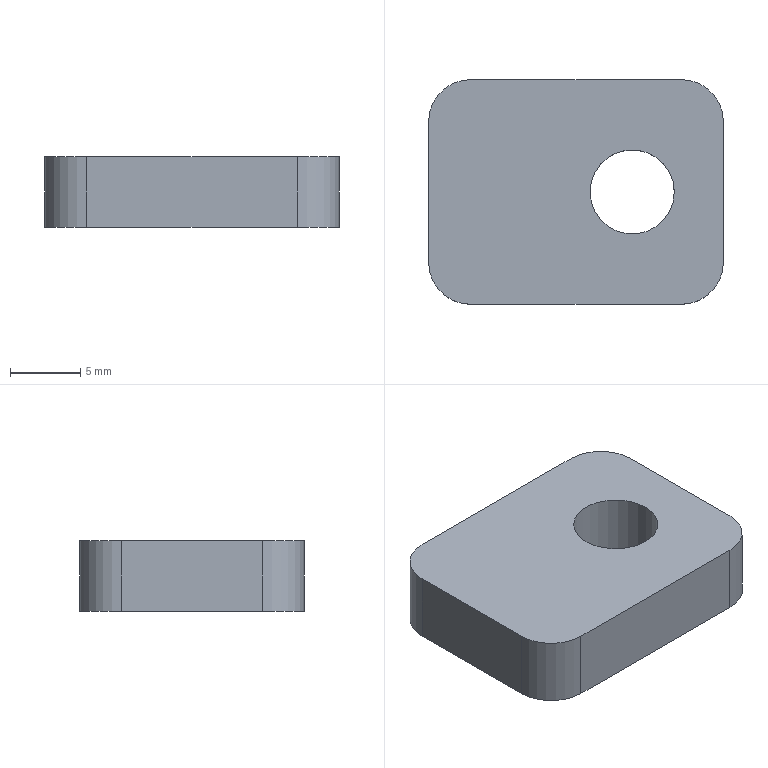Part | NX | features DIE-16 2 | 1 solid | 11 faces | box 21 x 16 x 5 mm | volume 1500 mm3 | plane 6 | cylinder 5 | commonest cylinder face diameters 6 x5
STEP:
#1=CARTESIAN_POINT('',(2415.893,-834.621,843.716));
#2=VERTEX_POINT('',#1);
#3=CARTESIAN_POINT('',(2415.893,-844.621,843.716));
#4=VERTEX_POINT('',#3);
#5=CARTESIAN_POINT('',(2415.893,-839.621,843.716));
#6=DIRECTION('',(0.,-1.,0.));
#7=VECTOR('',#6,1000.);
#8=LINE('',#5,#7);
#9=EDGE_CURVE('',#2,#4,#8,.T.);
#10=ORIENTED_EDGE('',*,*,#9,.F.);
#11=CARTESIAN_POINT('',(2415.893,-834.621,838.716));
#12=VERTEX_POINT('',#11);
#13=CARTESIAN_POINT('',(2415.893,-834.621,838.716));
#14=DIRECTION('',(0.,0.,1.));
#15=VECTOR('',#14,1000.);
#16=LINE('',#13,#15);
#17=EDGE_CURVE('',#12,#2,#16,.T.);
#18=ORIENTED_EDGE('',*,*,#17,.F.);
#19=CARTESIAN_POINT('',(2415.893,-844.621,838.716));
#20=VERTEX_POINT('',#19);
#21=CARTESIAN_POINT('',(2415.893,-839.621,838.716));
#22=DIRECTION('',(0.,-1.,0.));
#23=VECTOR('',#22,1000.);
#24=LINE('',#21,#23);
#25=EDGE_CURVE('',#12,#20,#24,.T.);
#26=ORIENTED_EDGE('',*,*,#25,.T.);
#27=CARTESIAN_POINT('',(2415.893,-844.621,838.716));
#28=DIRECTION('',(0.,0.,1.));
#29=VECTOR('',#28,1000.);
#30=LINE('',#27,#29);
#31=EDGE_CURVE('',#20,#4,#30,.T.);
#32=ORIENTED_EDGE('',*,*,#31,.T.);
#33=EDGE_LOOP('',(#10,#18,#26,#32));
#34=FACE_BOUND('',#33,.T.);
#35=CARTESIAN_POINT('',(2415.893,-839.621,838.716));
#36=DIRECTION('',(-1.,0.,0.));
#37=DIRECTION('',(0.,0.,1.));
#38=AXIS2_PLACEMENT_3D('',#35,#36,#37);
#39=PLANE('',#38);
#40=ADVANCED_FACE('',(#34),#39,.T.);
#41=CARTESIAN_POINT('',(2418.893,-831.621,843.716));
#42=VERTEX_POINT('',#41);
#43=CARTESIAN_POINT('',(2418.893,-834.621,843.716));
#44=DIRECTION('',(0.,0.,-1.));
#45=DIRECTION('',(-1.,0.,0.));
#46=AXIS2_PLACEMENT_3D('',#43,#44,#45);
#47=CIRCLE('',#46,3.);
#48=EDGE_CURVE('',#2,#42,#47,.T.);
#49=ORIENTED_EDGE('',*,*,#48,.T.);
#50=CARTESIAN_POINT('',(2418.893,-831.621,838.716));
#51=VERTEX_POINT('',#50);
#52=CARTESIAN_POINT('',(2418.893,-831.621,838.716));
#53=DIRECTION('',(0.,0.,1.));
#54=VECTOR('',#53,1000.);
#55=LINE('',#52,#54);
#56=EDGE_CURVE('',#51,#42,#55,.T.);
#57=ORIENTED_EDGE('',*,*,#56,.F.);
#58=CARTESIAN_POINT('',(2418.893,-834.621,838.716));
#59=DIRECTION('',(0.,0.,-1.));
#60=DIRECTION('',(-1.,0.,0.));
#61=AXIS2_PLACEMENT_3D('',#58,#59,#60);
#62=CIRCLE('',#61,3.);
#63=EDGE_CURVE('',#12,#51,#62,.T.);
#64=ORIENTED_EDGE('',*,*,#63,.F.);
#65=ORIENTED_EDGE('',*,*,#17,.T.);
#66=EDGE_LOOP('',(#49,#57,#64,#65));
#67=FACE_BOUND('',#66,.T.);
#68=CARTESIAN_POINT('',(2418.893,-834.621,838.716));
#69=DIRECTION('',(0.,0.,1.));
#70=DIRECTION('',(1.,0.,0.));
#71=AXIS2_PLACEMENT_3D('',#68,#69,#70);
#72=CYLINDRICAL_SURFACE('',#71,3.);
#73=ADVANCED_FACE('',(#67),#72,.T.);
#74=CARTESIAN_POINT('',(2433.893,-831.621,843.716));
#75=VERTEX_POINT('',#74);
#76=CARTESIAN_POINT('',(2421.393,-831.621,843.716));
#77=DIRECTION('',(-1.,0.,0.));
#78=VECTOR('',#77,1000.);
#79=LINE('',#76,#78);
#80=EDGE_CURVE('',#75,#42,#79,.T.);
#81=ORIENTED_EDGE('',*,*,#80,.F.);
#82=CARTESIAN_POINT('',(2433.893,-831.621,838.716));
#83=VERTEX_POINT('',#82);
#84=CARTESIAN_POINT('',(2433.893,-831.621,838.716));
#85=DIRECTION('',(0.,0.,1.));
#86=VECTOR('',#85,1000.);
#87=LINE('',#84,#86);
#88=EDGE_CURVE('',#83,#75,#87,.T.);
#89=ORIENTED_EDGE('',*,*,#88,.F.);
#90=CARTESIAN_POINT('',(2421.393,-831.621,838.716));
#91=DIRECTION('',(-1.,0.,0.));
#92=VECTOR('',#91,1000.);
#93=LINE('',#90,#92);
#94=EDGE_CURVE('',#83,#51,#93,.T.);
#95=ORIENTED_EDGE('',*,*,#94,.T.);
#96=ORIENTED_EDGE('',*,*,#56,.T.);
#97=EDGE_LOOP('',(#81,#89,#95,#96));
#98=FACE_BOUND('',#97,.T.);
#99=CARTESIAN_POINT('',(2421.393,-831.621,838.716));
#100=DIRECTION('',(0.,1.,0.));
#101=DIRECTION('',(0.,0.,1.));
#102=AXIS2_PLACEMENT_3D('',#99,#100,#101);
#103=PLANE('',#102);
#104=ADVANCED_FACE('',(#98),#103,.T.);
#105=CARTESIAN_POINT('',(2436.893,-834.621,843.716));
#106=VERTEX_POINT('',#105);
#107=CARTESIAN_POINT('',(2433.893,-834.621,843.716));
#108=DIRECTION('',(0.,0.,-1.));
#109=DIRECTION('',(-1.,0.,0.));
#110=AXIS2_PLACEMENT_3D('',#107,#108,#109);
#111=CIRCLE('',#110,3.);
#112=EDGE_CURVE('',#75,#106,#111,.T.);
#113=ORIENTED_EDGE('',*,*,#112,.T.);
#114=CARTESIAN_POINT('',(2436.893,-834.621,838.716));
#115=VERTEX_POINT('',#114);
#116=CARTESIAN_POINT('',(2436.893,-834.621,838.716));
#117=DIRECTION('',(0.,0.,1.));
#118=VECTOR('',#117,1000.);
#119=LINE('',#116,#118);
#120=EDGE_CURVE('',#115,#106,#119,.T.);
#121=ORIENTED_EDGE('',*,*,#120,.F.);
#122=CARTESIAN_POINT('',(2433.893,-834.621,838.716));
#123=DIRECTION('',(0.,0.,-1.));
#124=DIRECTION('',(-1.,0.,0.));
#125=AXIS2_PLACEMENT_3D('',#122,#123,#124);
#126=CIRCLE('',#125,3.);
#127=EDGE_CURVE('',#83,#115,#126,.T.);
#128=ORIENTED_EDGE('',*,*,#127,.F.);
#129=ORIENTED_EDGE('',*,*,#88,.T.);
#130=EDGE_LOOP('',(#113,#121,#128,#129));
#131=FACE_BOUND('',#130,.T.);
#132=CARTESIAN_POINT('',(2433.893,-834.621,838.716));
#133=DIRECTION('',(0.,0.,1.));
#134=DIRECTION('',(1.,0.,0.));
#135=AXIS2_PLACEMENT_3D('',#132,#133,#134);
#136=CYLINDRICAL_SURFACE('',#135,3.);
#137=ADVANCED_FACE('',(#131),#136,.T.);
#138=CARTESIAN_POINT('',(2436.893,-844.621,843.716));
#139=VERTEX_POINT('',#138);
#140=CARTESIAN_POINT('',(2436.893,-839.621,843.716));
#141=DIRECTION('',(0.,1.,0.));
#142=VECTOR('',#141,1000.);
#143=LINE('',#140,#142);
#144=EDGE_CURVE('',#139,#106,#143,.T.);
#145=ORIENTED_EDGE('',*,*,#144,.F.);
#146=CARTESIAN_POINT('',(2436.893,-844.621,838.716));
#147=VERTEX_POINT('',#146);
#148=CARTESIAN_POINT('',(2436.893,-844.621,838.716));
#149=DIRECTION('',(0.,0.,1.));
#150=VECTOR('',#149,1000.);
#151=LINE('',#148,#150);
#152=EDGE_CURVE('',#147,#139,#151,.T.);
#153=ORIENTED_EDGE('',*,*,#152,.F.);
#154=CARTESIAN_POINT('',(2436.893,-839.621,838.716));
#155=DIRECTION('',(0.,1.,0.));
#156=VECTOR('',#155,1000.);
#157=LINE('',#154,#156);
#158=EDGE_CURVE('',#147,#115,#157,.T.);
#159=ORIENTED_EDGE('',*,*,#158,.T.);
#160=ORIENTED_EDGE('',*,*,#120,.T.);
#161=EDGE_LOOP('',(#145,#153,#159,#160));
#162=FACE_BOUND('',#161,.T.);
#163=CARTESIAN_POINT('',(2436.893,-839.621,838.716));
#164=DIRECTION('',(1.,0.,0.));
#165=DIRECTION('',(0.,0.,-1.));
#166=AXIS2_PLACEMENT_3D('',#163,#164,#165);
#167=PLANE('',#166);
#168=ADVANCED_FACE('',(#162),#167,.T.);
#169=CARTESIAN_POINT('',(2433.893,-847.621,843.716));
#170=VERTEX_POINT('',#169);
#171=CARTESIAN_POINT('',(2433.893,-844.621,843.716));
#172=DIRECTION('',(0.,0.,-1.));
#173=DIRECTION('',(-1.,0.,0.));
#174=AXIS2_PLACEMENT_3D('',#171,#172,#173);
#175=CIRCLE('',#174,3.);
#176=EDGE_CURVE('',#139,#170,#175,.T.);
#177=ORIENTED_EDGE('',*,*,#176,.T.);
#178=CARTESIAN_POINT('',(2433.893,-847.621,838.716));
#179=VERTEX_POINT('',#178);
#180=CARTESIAN_POINT('',(2433.893,-847.621,838.716));
#181=DIRECTION('',(0.,0.,1.));
#182=VECTOR('',#181,1000.);
#183=LINE('',#180,#182);
#184=EDGE_CURVE('',#179,#170,#183,.T.);
#185=ORIENTED_EDGE('',*,*,#184,.F.);
#186=CARTESIAN_POINT('',(2433.893,-844.621,838.716));
#187=DIRECTION('',(0.,0.,-1.));
#188=DIRECTION('',(-1.,0.,0.));
#189=AXIS2_PLACEMENT_3D('',#186,#187,#188);
#190=CIRCLE('',#189,3.);
#191=EDGE_CURVE('',#147,#179,#190,.T.);
#192=ORIENTED_EDGE('',*,*,#191,.F.);
#193=ORIENTED_EDGE('',*,*,#152,.T.);
#194=EDGE_LOOP('',(#177,#185,#192,#193));
#195=FACE_BOUND('',#194,.T.);
#196=CARTESIAN_POINT('',(2433.893,-844.621,838.716));
#197=DIRECTION('',(0.,0.,1.));
#198=DIRECTION('',(1.,0.,0.));
#199=AXIS2_PLACEMENT_3D('',#196,#197,#198);
#200=CYLINDRICAL_SURFACE('',#199,3.);
#201=ADVANCED_FACE('',(#195),#200,.T.);
#202=CARTESIAN_POINT('',(2418.893,-847.621,843.716));
#203=VERTEX_POINT('',#202);
#204=CARTESIAN_POINT('',(2421.393,-847.621,843.716));
#205=DIRECTION('',(1.,0.,0.));
#206=VECTOR('',#205,1000.);
#207=LINE('',#204,#206);
#208=EDGE_CURVE('',#203,#170,#207,.T.);
#209=ORIENTED_EDGE('',*,*,#208,.F.);
#210=CARTESIAN_POINT('',(2418.893,-847.621,838.716));
#211=VERTEX_POINT('',#210);
#212=CARTESIAN_POINT('',(2418.893,-847.621,838.716));
#213=DIRECTION('',(0.,0.,1.));
#214=VECTOR('',#213,1000.);
#215=LINE('',#212,#214);
#216=EDGE_CURVE('',#211,#203,#215,.T.);
#217=ORIENTED_EDGE('',*,*,#216,.F.);
#218=CARTESIAN_POINT('',(2421.393,-847.621,838.716));
#219=DIRECTION('',(1.,0.,0.));
#220=VECTOR('',#219,1000.);
#221=LINE('',#218,#220);
#222=EDGE_CURVE('',#211,#179,#221,.T.);
#223=ORIENTED_EDGE('',*,*,#222,.T.);
#224=ORIENTED_EDGE('',*,*,#184,.T.);
#225=EDGE_LOOP('',(#209,#217,#223,#224));
#226=FACE_BOUND('',#225,.T.);
#227=CARTESIAN_POINT('',(2421.393,-847.621,838.716));
#228=DIRECTION('',(0.,-1.,0.));
#229=DIRECTION('',(0.,0.,-1.));
#230=AXIS2_PLACEMENT_3D('',#227,#228,#229);
#231=PLANE('',#230);
#232=ADVANCED_FACE('',(#226),#231,.T.);
#233=CARTESIAN_POINT('',(2427.393,-839.621,838.716));
#234=VERTEX_POINT('',#233);
#235=CARTESIAN_POINT('',(2430.393,-839.621,838.716));
#236=DIRECTION('',(0.,0.,-1.));
#237=DIRECTION('',(-1.,0.,0.));
#238=AXIS2_PLACEMENT_3D('',#235,#236,#237);
#239=CIRCLE('',#238,3.);
#240=EDGE_CURVE('',#234,#234,#239,.T.);
#241=ORIENTED_EDGE('',*,*,#240,.T.);
#242=EDGE_LOOP('',(#241));
#243=FACE_BOUND('',#242,.T.);
#244=CARTESIAN_POINT('',(2427.393,-839.621,843.716));
#245=VERTEX_POINT('',#244);
#246=CARTESIAN_POINT('',(2430.393,-839.621,843.716));
#247=DIRECTION('',(0.,0.,-1.));
#248=DIRECTION('',(-1.,0.,0.));
#249=AXIS2_PLACEMENT_3D('',#246,#247,#248);
#250=CIRCLE('',#249,3.);
#251=EDGE_CURVE('',#245,#245,#250,.T.);
#252=ORIENTED_EDGE('',*,*,#251,.F.);
#253=EDGE_LOOP('',(#252));
#254=FACE_BOUND('',#253,.T.);
#255=CARTESIAN_POINT('',(2430.393,-839.621,838.716));
#256=DIRECTION('',(0.,0.,1.));
#257=DIRECTION('',(1.,0.,0.));
#258=AXIS2_PLACEMENT_3D('',#255,#256,#257);
#259=CYLINDRICAL_SURFACE('',#258,3.);
#260=ADVANCED_FACE('',(#243,#254),#259,.F.);
#261=CARTESIAN_POINT('',(2418.893,-844.621,843.716));
#262=DIRECTION('',(0.,0.,-1.));
#263=DIRECTION('',(-1.,0.,0.));
#264=AXIS2_PLACEMENT_3D('',#261,#262,#263);
#265=CIRCLE('',#264,3.);
#266=EDGE_CURVE('',#203,#4,#265,.T.);
#267=ORIENTED_EDGE('',*,*,#266,.T.);
#268=ORIENTED_EDGE('',*,*,#31,.F.);
#269=CARTESIAN_POINT('',(2418.893,-844.621,838.716));
#270=DIRECTION('',(0.,0.,-1.));
#271=DIRECTION('',(-1.,0.,0.));
#272=AXIS2_PLACEMENT_3D('',#269,#270,#271);
#273=CIRCLE('',#272,3.);
#274=EDGE_CURVE('',#211,#20,#273,.T.);
#275=ORIENTED_EDGE('',*,*,#274,.F.);
#276=ORIENTED_EDGE('',*,*,#216,.T.);
#277=EDGE_LOOP('',(#267,#268,#275,#276));
#278=FACE_BOUND('',#277,.T.);
#279=CARTESIAN_POINT('',(2418.893,-844.621,838.716));
#280=DIRECTION('',(0.,0.,1.));
#281=DIRECTION('',(1.,0.,0.));
#282=AXIS2_PLACEMENT_3D('',#279,#280,#281);
#283=CYLINDRICAL_SURFACE('',#282,3.);
#284=ADVANCED_FACE('',(#278),#283,.T.);
#285=ORIENTED_EDGE('',*,*,#240,.F.);
#286=EDGE_LOOP('',(#285));
#287=FACE_BOUND('',#286,.T.);
#288=ORIENTED_EDGE('',*,*,#25,.F.);
#289=ORIENTED_EDGE('',*,*,#63,.T.);
#290=ORIENTED_EDGE('',*,*,#94,.F.);
#291=ORIENTED_EDGE('',*,*,#127,.T.);
#292=ORIENTED_EDGE('',*,*,#158,.F.);
#293=ORIENTED_EDGE('',*,*,#191,.T.);
#294=ORIENTED_EDGE('',*,*,#222,.F.);
#295=ORIENTED_EDGE('',*,*,#274,.T.);
#296=EDGE_LOOP('',(#288,#289,#290,#291,#292,#293,#294,#295));
#297=FACE_BOUND('',#296,.T.);
#298=CARTESIAN_POINT('',(2421.393,-839.621,838.716));
#299=DIRECTION('',(0.,0.,-1.));
#300=DIRECTION('',(-1.,0.,0.));
#301=AXIS2_PLACEMENT_3D('',#298,#299,#300);
#302=PLANE('',#301);
#303=ADVANCED_FACE('',(#287,#297),#302,.T.);
#304=ORIENTED_EDGE('',*,*,#251,.T.);
#305=EDGE_LOOP('',(#304));
#306=FACE_BOUND('',#305,.T.);
#307=ORIENTED_EDGE('',*,*,#9,.T.);
#308=ORIENTED_EDGE('',*,*,#266,.F.);
#309=ORIENTED_EDGE('',*,*,#208,.T.);
#310=ORIENTED_EDGE('',*,*,#176,.F.);
#311=ORIENTED_EDGE('',*,*,#144,.T.);
#312=ORIENTED_EDGE('',*,*,#112,.F.);
#313=ORIENTED_EDGE('',*,*,#80,.T.);
#314=ORIENTED_EDGE('',*,*,#48,.F.);
#315=EDGE_LOOP('',(#307,#308,#309,#310,#311,#312,#313,#314));
#316=FACE_BOUND('',#315,.T.);
#317=CARTESIAN_POINT('',(2421.393,-839.621,843.716));
#318=DIRECTION('',(0.,0.,-1.));
#319=DIRECTION('',(-1.,0.,0.));
#320=AXIS2_PLACEMENT_3D('',#317,#318,#319);
#321=PLANE('',#320);
#322=ADVANCED_FACE('',(#306,#316),#321,.F.);
#323=CLOSED_SHELL('',(#40,#73,#104,#137,#168,#201,#232,#260,#284,#303,#322));
#324=MANIFOLD_SOLID_BREP('',#323);
#325=(LENGTH_UNIT()NAMED_UNIT(*)SI_UNIT(.MILLI.,.METRE.));
#326=UNCERTAINTY_MEASURE_WITH_UNIT(LENGTH_MEASURE(0.00001),#325,'','');
#327=(NAMED_UNIT(*)PLANE_ANGLE_UNIT()SI_UNIT($,.RADIAN.));
#328=(NAMED_UNIT(*)SI_UNIT($,.STERADIAN.)SOLID_ANGLE_UNIT());
#329=(GEOMETRIC_REPRESENTATION_CONTEXT(3)GLOBAL_UNCERTAINTY_ASSIGNED_CONTEXT((#326))GLOBAL_UNIT_ASSIGNED_CONTEXT((#325,#327,#328))REPRESENTATION_CONTEXT('',''));
#330=ADVANCED_BREP_SHAPE_REPRESENTATION('',(#324),#329);